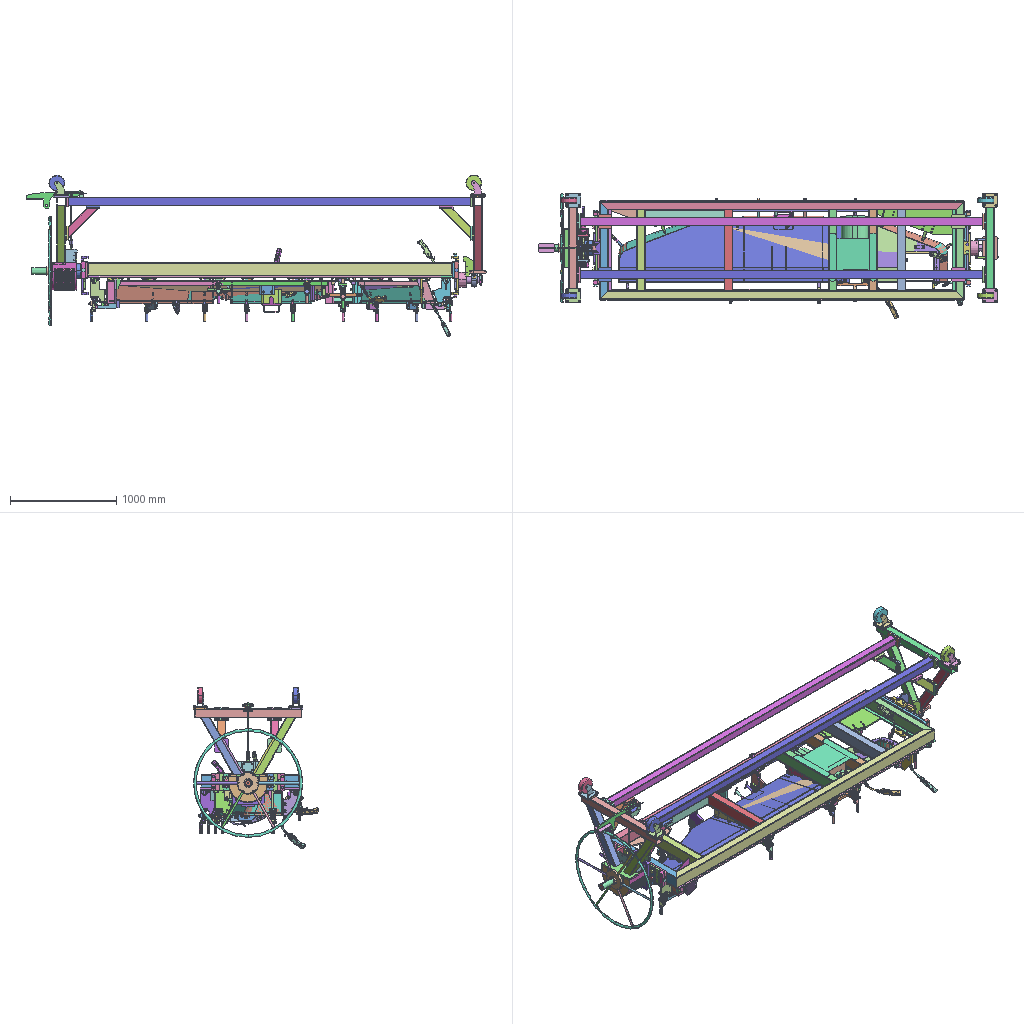Assembly | STEP file | 222 different items | 1217 placed | box 4334 x 1180 x 1526 mm
Parts list (item | name | quantity | parent item | size | volume):
1 | 01580-01008_1 | x3 | in ESTUDO-25-08-2019 | 19.63 x 17 x 8 mm | 1548 mm3
2 | 01580-01210_1 | x6 | in ESTUDO-25-08-2019 | 19 x 16.865 x 24.032 mm | 2301 mm3
3 | 09463-00005 | x2 | in ESTUDO-25-08-2019 | 20 x 31.754 x 24.699 mm | 4058 mm3
4 | 40A-00209-15-01 | x7 | in ESTUDO-25-08-2019 | 81.132 x 177.109 x 53.258 mm | 148559 mm3
5 | 40A-00285-23-03 | x1 | in ESTUDO-25-08-2019 | 3481 x 686 x 160 mm | 4684657 mm3
6 | 40A-00290-00-01-01 | x2 | in ESTUDO-25-08-2019 | 80 x 399.282 x 534.777 mm | 587215 mm3
7 | 40A-00290-00-01-01_INST | x2 | in ESTUDO-25-08-2019 | 80 x 447.282 x 617.915 mm | 679055 mm3
8 | 40A-00290-0020 | x2 | in ESTUDO-25-08-2019 | 80 x 1000 x 80 mm | 956670 mm3
9 | 40A-00290-005 | x1 | in ESTUDO-25-08-2019 | 100 x 83.152 x 47.419 mm | 122286 mm3
10 | 40A-00290-0050 | x1 | in ESTUDO-25-08-2019 | 450 x 450 x 4.25 mm | 726809 mm3
11 | 40A-00290-0050-01 | x1 | in ESTUDO-25-08-2019 | 227.055 x 4.25 x 163.4 mm | 122276 mm3
12 | 40A-00290-01-01 | x4 | in ESTUDO-25-08-2019 | 80 x 920 x 120 mm | 1480302 mm3
13 | 40A-00290-01-05 | x1 | in ESTUDO-25-08-2019 | 3316 x 940 x 14 mm | 15103628 mm3
14 | 40A-00290-01-06 | x5 | in ESTUDO-25-08-2019 | 80 x 760 x 120 mm | 1339263 mm3
15 | 40A-00290-01-09 | x1 | in ESTUDO-25-08-2019 | 150 x 12.7 x 80 mm | 90011 mm3
16 | 40A-00290-01-10 | x1 | in ESTUDO-25-08-2019 | 745 x 80 x 120 mm | 1312830 mm3
17 | 40A-00290-01-12 | x2 | in ESTUDO-25-08-2019 | 74 x 4.7 x 115 mm | 39912 mm3
18 | 40A-00290-02 | x3 | in ESTUDO-25-08-2019 | 22.2 x 550 x 100.58 mm | 539810 mm3
19 | 40A-00290-03 | x292 | in ESTUDO-25-08-2019 | 20 x 40 x 0.9 mm | 598.289 mm3
20 | 40A-00290-04 | x6 | in ESTUDO-25-08-2019 | 1059 x 97.075 x 221.8 mm | 15871 mm3
21 | 40A-00290-05 | x2 | in ESTUDO-25-08-2019 | 22.2 x 330 x 53.73 mm | 174983 mm3
22 | 40A-00290-06-01 | x1 | in ESTUDO-25-08-2019 | 80 x 115 x 17 mm | 142679 mm3
23 | 40A-00290-06-02 | x1 | in ESTUDO-25-08-2019 | 130 x 19.05 x 222.5 mm | 357231 mm3
24 | 40A-00290-06-03 | x2 | in ESTUDO-25-08-2019 | 9.5 x 30 x 80 mm | 18003 mm3
25 | 40A-00290-06-04 | x8 | in ESTUDO-25-08-2019 | 60 x 65 x 10 mm | 37467 mm3
26 | 40A-00290-07-01 | x1 | in ESTUDO-25-08-2019 | 178.5 x 22.2 x 49.5 mm | 141858 mm3
27 | 40A-00290-08 | x12 | in ESTUDO-25-08-2019 | 22.2 x 25 x 24.5 mm | 8372 mm3
28 | 40A-00290-09 | x12 | in ESTUDO-25-08-2019 | 22.2 x 25 x 18 mm | 5554 mm3
29 | 40A-00290-090-01 | x8 | in ESTUDO-25-08-2019 | 14 x 150 x 100 mm | 207200 mm3
30 | 40A-00290-090-02 | x4 | in ESTUDO-25-08-2019 | 140 x 130 x 14 mm | 252000 mm3
31 | 40A-00290-091-02 | x2 | in ESTUDO-25-08-2019 | 3792 x 80 x 80 mm | 3627596 mm3
32 | 40A-00290-091-04 | x1 | in ESTUDO-25-08-2019 | 14 x 150 x 60 mm | 123200 mm3
33 | 40A-00290-092-03 | x4 | in ESTUDO-25-08-2019 | 285.105 x 80 x 285.105 mm | 306135 mm3
34 | 40A-00290-092-05 | x16 | in ESTUDO-25-08-2019 | 14 x 130 x 130 mm | 233800 mm3
35 | 40A-00290-10 | x8 | in ESTUDO-25-08-2019 | 20 x 20 x 70 mm | 25167 mm3
36 | 40A-00290-11 | x8 | in ESTUDO-25-08-2019 | 70 x 20 x 17 mm | 15529 mm3
37 | 40A-00290-12 | x40 | in ESTUDO-25-08-2019 | 70 x 20 x 0.9 mm | 1138 mm3
38 | 40A-00290-13-01 | x7 | in ESTUDO-25-08-2019 | 139.849 x 121.618 x 17.086 mm | 169879 mm3
39 | 40A-00290-13-02 | x7 | in ESTUDO-25-08-2019 | 76.391 x 163.749 x 226.519 mm | 512564 mm3
40 | 40A-00290-13-03 | x8 | in ESTUDO-25-08-2019 | 36.194 x 20.702 x 100.009 mm | 28387 mm3
41 | 40A-00290-14 | x7 | in ESTUDO-25-08-2019 | 30.891 x 43.057 x 18.238 mm | 8045 mm3
42 | 40A-00290-16-01 | x1 | in ESTUDO-25-08-2019 | 130 x 90.001 x 20.006 mm | 217858 mm3
43 | 40A-00290-16-02 | x1 | in ESTUDO-25-08-2019 | 22.2 x 252.412 x 220.3 mm | 586944 mm3
44 | 40A-00290-16-04 | x1 | in ESTUDO-25-08-2019 | 65 x 55.001 x 12.004 mm | 41061 mm3
45 | 40A-00290-17-01 | x1 | in ESTUDO-25-08-2019 | 100 x 160.002 x 37.06 mm | 154063 mm3
46 | 40A-00290-18 | x4 | in ESTUDO-25-08-2019 | 20 x 60.001 x 17.004 mm | 14302 mm3
47 | 40A-00290-21-01 | x1 | in ESTUDO-25-08-2019 | 115 x 70 x 17 mm | 123129 mm3
48 | 40A-00290-21-02 | x1 | in ESTUDO-25-08-2019 | 19.05 x 130 x 229.5 mm | 353478 mm3
49 | 40A-00290-21-04 | x1 | in ESTUDO-25-08-2019 | 21 x 10 x 50 mm | 9323 mm3
50 | 40A-00290-22 | x2 | in ESTUDO-25-08-2019 | 20 x 17 x 65 mm | 14789 mm3
51 | 40A-00290-23-01 | x1 | in ESTUDO-25-08-2019 | 120 x 80 x 17 mm | 149479 mm3
52 | 40A-00290-23-02 | x1 | in ESTUDO-25-08-2019 | 22.2 x 125 x 112.6 mm | 155694 mm3
53 | 40A-00290-23-03 | x1 | in ESTUDO-25-08-2019 | 35 x 9.5 x 45 mm | 10100 mm3
54 | 40A-00290-23-04 | x2 | in ESTUDO-25-08-2019 | 65 x 55 x 10 mm | 34217 mm3
55 | 40A-00290-24-01 | x1 | in ESTUDO-25-08-2019 | 325 x 165 x 25.4 mm | 302458 mm3
56 | 40A-00290-27 | x1 | in ESTUDO-25-08-2019 | 15 x 15 x 28 mm | 3220 mm3
57 | 40A-00290-31-01 | x2 | in ESTUDO-25-08-2019 | 130 x 100 x 17 mm | 207279 mm3
58 | 40A-00290-31-02 | x1 | in ESTUDO-25-08-2019 | 22.2 x 65 x 59 mm | 66200 mm3
59 | 40A-00290-32-01 | x1 | in ESTUDO-25-08-2019 | 25.4 x 163 x 75 mm | 143731 mm3
60 | 40A-00290-33 | x3 | in ESTUDO-25-08-2019 | 15 x 25.4 x 25.4 mm | 5795 mm3
61 | 40A-00290-34 | x15 | in ESTUDO-25-08-2019 | 0.9 x 25.4 x 25.4 mm | 398.781 mm3
62 | 40A-00290-35-01 | x1 | in ESTUDO-25-08-2019 | 220 x 163 x 25.4 mm | 220844 mm3
63 | 40A-00290-35-02 | x2 | in ESTUDO-25-08-2019 | 25.4 x 35 x 50 mm | 40932 mm3
64 | 40A-00290-36-02 | x1 | in ESTUDO-25-08-2019 | 22.2 x 65 x 63.6 mm | 71314 mm3
65 | 40A-00290-36-03 | x1 | in ESTUDO-25-08-2019 | 64 x 55 x 10 mm | 33667 mm3
66 | 40A-00290-37-01 | x1 | in ESTUDO-25-08-2019 | 120 x 70 x 17 mm | 129079 mm3
67 | 40A-00290-37-02 | x1 | in ESTUDO-25-08-2019 | 19.05 x 130 x 229.5 mm | 352712 mm3
68 | 40A-00290-37-03 | x1 | in ESTUDO-25-08-2019 | 30 x 9.5 x 90 mm | 20853 mm3
69 | 40A-00290-38 | x1 | in ESTUDO-25-08-2019 | 3521 x 545 x 260 mm | 4239182 mm3
70 | 40A-00290-39 | x1 | in ESTUDO-25-08-2019 | 3559 x 300 x 364.4 mm | 4151060 mm3
71 | 40A-00290-40 | x2 | in ESTUDO-25-08-2019 | 3557 x 686 x 160 mm | 380275 mm3
72 | 40A-00290-41 | x4 | in ESTUDO-25-08-2019 | 4.7 x 63.5 x 160 mm | 42903 mm3
73 | 40A-00290-43-01 | x1 | in ESTUDO-25-08-2019 | 3214 x 169.325 x 80 mm | 319398 mm3
74 | 40A-00290-43-02 | x2 | in ESTUDO-25-08-2019 | 39.146 x 39.199 x 25.4 mm | 10583 mm3
75 | 40A-00290-44 | x2 | in ESTUDO-25-08-2019 | 108.959 x 110.316 x 27.713 mm | 32998 mm3
76 | 40A-00290-45 | x1 | in ESTUDO-25-08-2019 | 80 x 22.2 x 32.7 mm | 46344 mm3
77 | 40A-00290-46 | x1 | in ESTUDO-25-08-2019 | 34.62 x 34.745 x 53 mm | 22336 mm3
78 | 40A-00290-47 | x1 | in ESTUDO-25-08-2019 | 35.533 x 31.929 x 53 mm | 22916 mm3
79 | 40A-00290-48-01 | x2 | in ESTUDO-25-08-2019 | 85 x 22.827 x 45.038 mm | 25290 mm3
80 | 40A-00290-48-02 | x2 | in ESTUDO-25-08-2019 | 9.5 x 91.862 x 99.473 mm | 32858 mm3
81 | 40A-00290-48-03 | x4 | in ESTUDO-25-08-2019 | 15 x 24.154 x 18.477 mm | 2911 mm3
82 | 40A-00290-49-01 | x1 | in ESTUDO-25-08-2019 | 190 x 54.37 x 130.354 mm | 253726 mm3
83 | 40A-00290-49-02 | x1 | in ESTUDO-25-08-2019 | 153 x 43.131 x 103.161 mm | 17399 mm3
84 | 40A-00290-50 | x2 | in ESTUDO-25-08-2019 | 22.2 x 156.403 x 95.773 mm | 46590 mm3
85 | 40A-00290-52 | x1 | in ESTUDO-25-08-2019 | 85 x 140 x 140 mm | 891287 mm3
86 | 40A-00290-53 | x1 | in ESTUDO-25-08-2019 | 484.5 x 62.198 x 63.5 mm | 1142527 mm3
87 | 40A-00290-56 | x1 | in ESTUDO-25-08-2019 | 139.5 x 61.15 x 61.15 mm | 51845 mm3
88 | 40A-00290-57 | x1 | in ESTUDO-25-08-2019 | 8 x 63.5 x 63.5 mm | 24378 mm3
89 | 40A-00290-58-01 | x1 | in ESTUDO-25-08-2019 | 25.4 x 1025 x 1025 mm | 1591868 mm3
90 | 40A-00290-58-02 | x1 | in ESTUDO-25-08-2019 | 45.4 x 200 x 200 mm | 794130 mm3
91 | 40A-00290-58-03 | x3 | in ESTUDO-25-08-2019 | 19.05 x 447.696 x 434.908 mm | 222589 mm3
92 | 40A-00290-59 | x1 | in ESTUDO-25-08-2019 | 14 x 198.529 x 198.529 mm | 329948 mm3
93 | 40A-00290-60 | x1 | in ESTUDO-25-08-2019 | 37 x 37 x 174 mm | 65874 mm3
94 | 40A-00290-61-01 | x1 | in ESTUDO-25-08-2019 | 10 x 100 x 78 mm | 75275 mm3
95 | 40A-00290-61-02 | x1 | in ESTUDO-25-08-2019 | 63.5 x 63.5 x 88 mm | 177757 mm3
96 | 40A-00290-62 | x1 | in ESTUDO-25-08-2019 | 63.5 x 63.5 x 15 mm | 31384 mm3
97 | 40A-00290-63 | x1 | in ESTUDO-25-08-2019 | 25.4 x 25.4 x 496.8 mm | 47763 mm3
98 | 40A-00290-64 | x1 | in ESTUDO-25-08-2019 | 10 x 10 x 411.8 mm | 32313 mm3
99 | 40A-00290-65 | x2 | in ESTUDO-25-08-2019 | 8 x 38 x 8 mm | 1837 mm3
100 | 40A-00290-66-01 | x1 | in ESTUDO-25-08-2019 | 10 x 130 x 50 mm | 61955 mm3
101 | 40A-00290-66-02 | x2 | in ESTUDO-25-08-2019 | 150 x 9.53 x 120 mm | 89007 mm3
102 | 40A-00290-66-03 | x1 | in ESTUDO-25-08-2019 | 150 x 51 x 9.5 mm | 62585 mm3
103 | 40A-00290-67 | x1 | in ESTUDO-25-08-2019 | 16 x 95 x 16 mm | 18654 mm3
104 | 40A-00290-68-01 | x1 | in ESTUDO-25-08-2019 | 513 x 9.53 x 163.52 mm | 271409 mm3
105 | 40A-00290-68-02 | x1 | in ESTUDO-25-08-2019 | 38.1 x 50 x 38.1 mm | 46834 mm3
106 | 40A-00290-68-03 | x2 | in ESTUDO-25-08-2019 | 140 x 15 x 9.53 mm | 13647 mm3
107 | 40A-00290-68-04 | x1 | in ESTUDO-25-08-2019 | 160 x 90 x 9.53 mm | 135326 mm3
108 | 40A-00290-72 | x1 | in ESTUDO-25-08-2019 | 175 x 70 x 115 mm | 354773 mm3
109 | 40A-00290-73-01 | x1 | in ESTUDO-25-08-2019 | 65 x 8 x 98 mm | 32438 mm3
110 | 40A-00290-73-02 | x1 | in ESTUDO-25-08-2019 | 50.8 x 84 x 50.8 mm | 109071 mm3
111 | 40A-00290-74 | x1 | in ESTUDO-25-08-2019 | 30 x 264 x 100 mm | 106640 mm3
112 | 40A-00290-75 | x1 | in ESTUDO-25-08-2019 | 52 x 53 x 52 mm | 27030 mm3
113 | 40A-00290-76 | x1 | in ESTUDO-25-08-2019 | 12.7 x 265 x 185 mm | 468298 mm3
114 | 40A-00290-77 | x2 | in ESTUDO-25-08-2019 | 5 x 65 x 65 mm | 4712 mm3
115 | 40A-00290-78-01 | x1 | in ESTUDO-25-08-2019 | 237 x 366.4 x 268.2 mm | 401444 mm3
116 | 40A-00290-78-02 | x1 | in ESTUDO-25-08-2019 | 3.2 x 360 x 265 mm | 131424 mm3
117 | 40A-00290-78-03 | x1 | in ESTUDO-25-08-2019 | 3.2 x 360 x 265 mm | 148242 mm3
118 | 40A-00290-79-03 | x1 | in ESTUDO-25-08-2019 | 130 x 360 x 20 mm | 917624 mm3
119 | 40A-00290-79-04 | x2 | in ESTUDO-25-08-2019 | 111 x 19.05 x 150 mm | 264775 mm3
120 | 40A-00290-79-05 | x1 | in ESTUDO-25-08-2019 | 15.88 x 220 x 95 mm | 305176 mm3
121 | 40A-00290-80-03 | x1 | in ESTUDO-25-08-2019 | 150 x 220 x 23 mm | 740391 mm3
122 | 40A-00290-80-04 | x2 | in ESTUDO-25-08-2019 | 97 x 19.05 x 188 mm | 224264 mm3
123 | 40A-00290-83 | x1 | in ESTUDO-25-08-2019 | 70 x 140 x 140 mm | 753784 mm3
124 | 40A-00290-84 | x1 | in ESTUDO-25-08-2019 | 92 x 11 x 18 mm | 17898 mm3
125 | 40A-00290-85 | x1 | in ESTUDO-25-08-2019 | 243 x 62.198 x 63.5 mm | 632227 mm3
126 | 40A-00290-86 | x1 | in ESTUDO-25-08-2019 | 19.05 x 95 x 86 mm | 87313 mm3
127 | 4A2-54-11L10 | x1 | in ESTUDO-25-08-2019 | 3098 x 622.4 x 213.706 mm | 2369669 mm3
128 | 4A2-54-11L11_1 | x1 | in ESTUDO-25-08-2019 | 3098 x 622.4 x 213.7 mm | 2346109 mm3
129 | 4A2-54-11L20 | x1 | in ESTUDO-25-08-2019 | 2166 x 577 x 97.501 mm | 5121201 mm3
130 | 4A2-54-11L21_1 | x1 | in ESTUDO-25-08-2019 | 2121 x 577 x 97.501 mm | 5018466 mm3
131 | 4A2-54-11L30 | x1 | in ESTUDO-25-08-2019 | 741.47 x 576.675 x 97.432 mm | 1088545 mm3
132 | 4A2-54-11L31_1 | x1 | in ESTUDO-25-08-2019 | 698.953 x 565.957 x 95.154 mm | 991913 mm3
133 | 4A2-54-11L40 | x1 | in ESTUDO-25-08-2019 | 2132 x 611.11 x 209.3 mm | 740034 mm3
134 | 4A2-54-11L41_1 | x1 | in ESTUDO-25-08-2019 | 2074 x 4.5 x 209.3 mm | 441896 mm3
135 | 4A2-54-11L50 | x1 | in ESTUDO-25-08-2019 | 774.723 x 599.917 x 209.3 mm | 695690 mm3
136 | 4A2-54-11L51_1 | x1 | in ESTUDO-25-08-2019 | 719.279 x 4.5 x 209.3 mm | 189254 mm3
137 | 4A2-54-11L60 | x2 | in ESTUDO-25-08-2019 | 32 x 35 x 32 mm | 33597 mm3
138 | 4A2-54-11L70_1 | x3 | in ESTUDO-25-08-2019 | 4.5 x 606.608 x 209.3 mm | 136456 mm3
139 | 4A2-54-11L80 | x1 | in ESTUDO-25-08-2019 | 992.7 x 598.55 x 4.5 mm | 515371 mm3
140 | 4A2-54-11L81_1 | x1 | in ESTUDO-25-08-2019 | 992.7 x 598.55 x 4.5 mm | 514819 mm3
141 | 4A2-54-11L90 | x1 | in ESTUDO-25-08-2019 | 738.135 x 582.284 x 4.5 mm | 405485 mm3
142 | 4A2-54-11L91_1 | x1 | in ESTUDO-25-08-2019 | 729.149 x 582.284 x 4.5 mm | 403195 mm3
143 | 4A2-54-11M10 | x1 | in ESTUDO-25-08-2019 | 190 x 43.445 x 109.958 mm | 50702 mm3
144 | 4A2-54-11M11_1 | x1 | in ESTUDO-25-08-2019 | 190 x 43.445 x 108.427 mm | 50431 mm3
145 | 4A2-54-11M20 | x2 | in ESTUDO-25-08-2019 | 190 x 118.6 x 132.5 mm | 194744 mm3
146 | 4A2-54-11M30_1 | x2 | in ESTUDO-25-08-2019 | 273 x 90 x 4.5 mm | 110403 mm3
147 | 4A2-54-11M50 | x1 | in ESTUDO-25-08-2019 | 247 x 124.327 x 38 mm | 141414 mm3
148 | 4A2-54-11M51_1 | x1 | in ESTUDO-25-08-2019 | 250.292 x 106.987 x 48.736 mm | 83398 mm3
149 | 4A2-54-11M60 | x1 | in ESTUDO-25-08-2019 | 250.111 x 140 x 4.5 mm | 148675 mm3
150 | 4A2-54-11M61_1 | x1 | in ESTUDO-25-08-2019 | 253.292 x 115 x 4.5 mm | 94907 mm3
151 | 4A2-54-11M70_1 | x1 | in ESTUDO-25-08-2019 | 316 x 281.468 x 37.023 mm | 104532 mm3
152 | 4A2-54-11M80_1 | x4 | in ESTUDO-25-08-2019 | 4.5 x 83.967 x 43.509 mm | 6250 mm3
153 | 4A2-54-11M90_1 | x1 | in ESTUDO-25-08-2019 | 90 x 32.255 x 19.931 mm | 36211 mm3
154 | 4A2-54-11N11_1 | x1 | in ESTUDO-25-08-2019 | 262 x 552 x 144.907 mm | 1122915 mm3
155 | 4A2-54-12C11_1 | x1 | in ESTUDO-25-08-2019 | 80 x 604.972 x 204.8 mm | 226498 mm3
156 | 4A2-54-12C20_1 | x1 | in ESTUDO-25-08-2019 | 80 x 594.996 x 209.3 mm | 492468 mm3
157 | 4A2-54-12D10_1 | x1 | in ESTUDO-25-08-2019 | 69 x 69 x 95.5 mm | 55112 mm3
158 | 4A2-54-12D20_1 | x1 | in ESTUDO-25-08-2019 | 75 x 75 x 4.5 mm | 24190 mm3
159 | 4A2-54-12D30_1 | x1 | in ESTUDO-25-08-2019 | 9 x 55 x 55 mm | 24913 mm3
160 | 4A2-54-12D40_1 | x1 | in ESTUDO-25-08-2019 | 32 x 25 x 105 mm | 79834 mm3
161 | 4A2-54-12E10_1 | x1 | in ESTUDO-25-08-2019 | 35 x 35 x 187 mm | 50638 mm3
162 | 4A2-54-12E20_1 | x1 | in ESTUDO-25-08-2019 | 40 x 40 x 4.5 mm | 6262 mm3
163 | 4A2-54-12E60_1 | x1 | in ESTUDO-25-08-2019 | 136 x 300 x 129.521 mm | 246784 mm3
164 | BEARING-UCP-211-KONTIMA_UCP_211 | x1 | in ESTUDO-25-08-2019 | 3966 x 100 x 184 mm | 353465 mm3
165 | CABECOTE_ | x4 | in ESTUDO-25-08-2019 | 140 x 130 x 138.61 mm | 251039 mm3
166 | COMERCIAL_DESTACO_GU5D-01 | x12 | in ESTUDO-25-08-2019 | 55 x 64 x 8 mm | 26280 mm3
167 | COMERCIAL_DESTACO_GU5D-03 | x12 | in ESTUDO-25-08-2019 | 22.22 x 22.221 x 79.977 mm | 12383 mm3
168 | COMERCIAL_DESTACO_GU5D-04 | x1 | in ESTUDO-25-08-2019 | 3406 x 811.269 x 242.561 mm | 328941 mm3
169 | COMERCIAL_DESTACO_GU5D-05 | x12 | in ESTUDO-25-08-2019 | 104.913 x 21.7 x 63.06 mm | 40442 mm3
170 | COMERCIAL_DESTACO_GU5D-06 | x12 | in ESTUDO-25-08-2019 | 25.534 x 21.4 x 66.7 mm | 14812 mm3
171 | COMERCIAL_DESTACO_GU5D-07 | x12 | in ESTUDO-25-08-2019 | 79.798 x 21.7 x 52.943 mm | 21756 mm3
172 | COMERCIAL_DESTACO_GU5D-08 | x12 | in ESTUDO-25-08-2019 | 35 x 12.3 x 45.5 mm | 17099 mm3
173 | COMERCIAL_DIN125A_17 | x2 | in ESTUDO-25-08-2019 | 30 x 3 x 30 mm | 1394 mm3
174 | COMERCIAL_DIN7979_16X50 | x2 | in ESTUDO-25-08-2019 | 50 x 16 x 16 mm | 10005 mm3
175 | COMERCIAL_DIN912-M20X45-MONT | x2 | in ESTUDO-25-08-2019 | 37 x 37 x 65 mm | 30629 mm3
176 | COMERCIAL_IGUS_GSM-2224-15 | x4 | in ESTUDO-25-08-2019 | 24 x 24 x 15 mm | 1055 mm3
177 | COMERCIAL_MAGNETICO | x38 | in ESTUDO-25-08-2019 | 16 x 16 x 10 mm | 2011 mm3
178 | COMERCIAL_TRIT_CL_5_BLPB2 | x2 | in ESTUDO-25-08-2019 | 47 x 28.5 x 28.5 mm | 5603 mm3
179 | DIN580-M16 | x4 | in ESTUDO-25-08-2019 | 44.167 x 52.613 x 89 mm | 37281 mm3
180 | DIN7979-08X24 | x2 | in ESTUDO-25-08-2019 | 8 x 8 x 24 mm | 1191 mm3
181 | DIN7979-08X55 | x1 | in ESTUDO-25-08-2019 | 8 x 8 x 55 mm | 2750 mm3
182 | DIN7979-10X30 | x4 | in ESTUDO-25-08-2019 | 10 x 10 x 30 mm | 2337 mm3
183 | DIN7979-10X35 | x6 | in ESTUDO-25-08-2019 | 10 x 10 x 35 mm | 2730 mm3
184 | DIN7979-12X35 | x28 | in ESTUDO-25-08-2019 | 12 x 12 x 35 mm | 3923 mm3
185 | DIN912-M10X35 | x10 | in ESTUDO-25-08-2019 | 16.3 x 16.3 x 45 mm | 4558 mm3
186 | DIN912-M10X45 | x2 | in ESTUDO-25-08-2019 | 16.3 x 16.3 x 55 mm | 5344 mm3
187 | DIN912-M10X55 | x6 | in ESTUDO-25-08-2019 | 16.3 x 16.3 x 65 mm | 6129 mm3
188 | DIN912-M12X30 | x2 | in ESTUDO-25-08-2019 | 3923 x 251.8 x 694.71 mm | 12059 mm3
189 | DIN912-M12X35 | x56 | in ESTUDO-25-08-2019 | 18.3 x 18.3 x 47 mm | 6595 mm3
190 | DIN912-M12X80 | x2 | in ESTUDO-25-08-2019 | 18.3 x 18.3 x 92 mm | 11684 mm3
191 | DIN912-M16X50 | x4 | in ESTUDO-25-08-2019 | 3553 x 672.2 x 24.3 mm | 32231 mm3
192 | DIN912-M16X70 | x4 | in ESTUDO-25-08-2019 | 86 x 24.3 x 24.3 mm | 20137 mm3
193 | DIN912-M5X20 | x4 | in ESTUDO-25-08-2019 | 8.7 x 25 x 8.7 mm | 655.292 mm3
194 | DIN912-M6X16 | x12 | in ESTUDO-25-08-2019 | 10.2 x 10.2 x 52 mm | 1755 mm3
195 | DIN912-M8X110 | x2 | in ESTUDO-25-08-2019 | 13.3 x 13.3 x 118 mm | 6516 mm3
196 | DIN912-M8X16 | x48 | in ESTUDO-25-08-2019 | 13.3 x 13.3 x 24 mm | 1791 mm3
197 | DIN912-M8X20 | x111 | in ESTUDO-25-08-2019 | 13.3 x 13.3 x 8 mm | 765.054 mm3
198 | DIN912-M8X25 | x36 | in ESTUDO-25-08-2019 | 33 x 13.3 x 13.3 mm | 2243 mm3
199 | DIN912-M8X25-12_9 | x5 | in ESTUDO-25-08-2019 | 13 x 20.166 x 34.272 mm | 2161 mm3
200 | DIN912-M8X35 | x2 | in ESTUDO-25-08-2019 | 392.763 x 335.773 x 13.82 mm | 5492 mm3
201 | DIN933-M16X70 | x2 | in ESTUDO-25-08-2019 | 27.713 x 24 x 420 mm | 38125 mm3
202 | DIN933-M20X70 | x2 | in ESTUDO-25-08-2019 | 3548 x 715.8 x 30 mm | 64247 mm3
203 | DIN933-M24X45 | x4 | in ESTUDO-25-08-2019 | 3560 x 36 x 121.569 mm | 74386 mm3
204 | DIN933-M8X16 | x1 | in ESTUDO-25-08-2019 | 25.531 x 13 x 90.006 mm | 3218 mm3
205 | DIN934-M10 | x2 | in ESTUDO-25-08-2019 | 17 x 19.63 x 8 mm | 1374 mm3
206 | DIN934-M16 | x4 | in ESTUDO-25-08-2019 | 24 x 27.713 x 13 mm | 3871 mm3
207 | DIN934-M20 | x4 | in ESTUDO-25-08-2019 | 30 x 16 x 34.641 mm | 7444 mm3
208 | DIN934-M8 | x2 | in ESTUDO-25-08-2019 | 13 x 15.011 x 6.5 mm | 624.603 mm3
209 | DIN_125A_M8 | x4 | in ESTUDO-25-08-2019 | 17 x 1.6 x 17 mm | 274.5 mm3
210 | DIN_94_2X16 | x4 | in ESTUDO-25-08-2019 | 3.6 x 1.8 x 22.5 mm | 54.298 mm3
211 | DIN_94_4X32 | x2 | in ESTUDO-25-08-2019 | 44 x 3.7 x 7.4 mm | 454.484 mm3
212 | HOUSE-UCP-211-KONTIMA_UCP_211-K | x2 | in ESTUDO-25-08-2019 | 60 x 219 x 126 mm | 386400 mm3
213 | ISO8734-8X30-C1 | x2 | in ESTUDO-25-08-2019 | 8 x 16.378 x 30.707 mm | 1491 mm3
214 | LUBRICATION-NIPPLE-UCP-211-KONT | x2 | in ESTUDO-25-08-2019 | 8.083 x 7 x 14.5 mm | 420.781 mm3
215 | RODA_ | x4 | in ESTUDO-25-08-2019 | 150 x 50 x 150 mm | 872054 mm3
216 | SPEC_MOLA_1-125-08-03 | x4 | in ESTUDO-25-08-2019 | 11.25 x 11.25 x 13.12 mm | 160.677 mm3
217 | SPEC_MOLA_1-400-10-03 | x1 | in ESTUDO-25-08-2019 | - | 9018 mm3
218 | SPEC_MOLA_12001205 | x1 | in ESTUDO-25-08-2019 | - | 2341 mm3
219 | TOCHA-1-SOLID1 | x3 | in ESTUDO-25-08-2019 | - | 28159 mm3
220 | TOCHA-1-SOLID2 | x6 | in ESTUDO-25-08-2019 | 11.133 x 47.566 x 27.63 mm | 1937 mm3
221 | TOCHA-1-SOLID3 | x1 | in ESTUDO-25-08-2019 | 2607 x 1013 x 916.163 mm | 1110873 mm3
222 | TOCHA-1-SOLID4 | x6 | in ESTUDO-25-08-2019 | 8.632 x 21.191 x 21.284 mm | 26.231 mm3